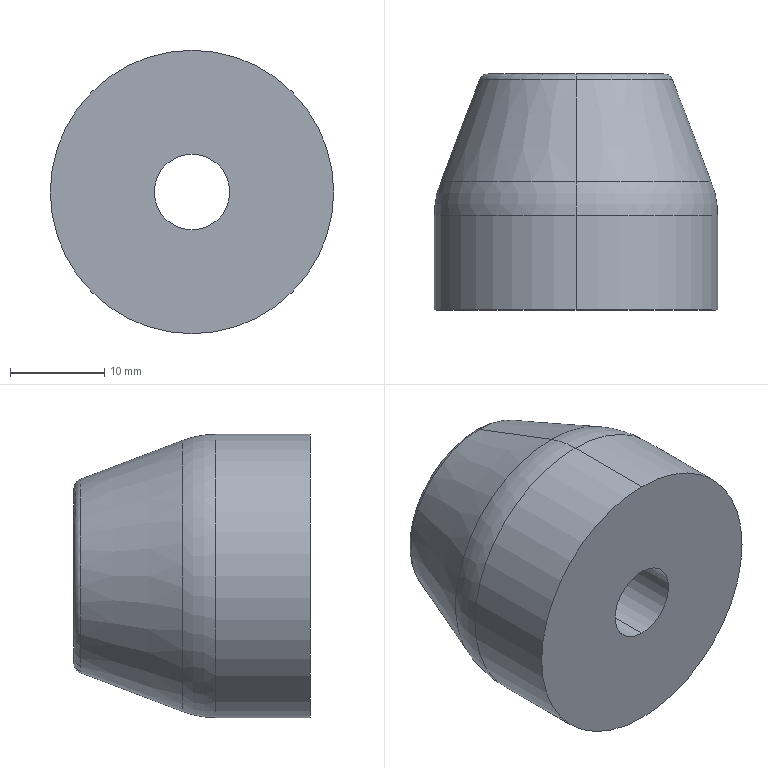Part | SolidWorks | features Revolution 1 | 1 solid | 15 faces | box 30 x 25 x 30 mm | volume 12754 mm3 | cylinder 6 | torus 4 | plane 3 | cone 2 | commonest cylinder face diameters 8 x2 12 x2 30 x2
STEP:
#1=CARTESIAN_POINT('',(0.,11.,4.));
#2=VERTEX_POINT('',#1);
#3=CARTESIAN_POINT('',(0.,11.,-4.));
#4=VERTEX_POINT('',#3);
#5=CARTESIAN_POINT('',(0.,11.,0.));
#6=DIRECTION('',(0.,-1.,0.));
#7=DIRECTION('',(0.,0.,-1.));
#8=AXIS2_PLACEMENT_3D('',#5,#6,#7);
#9=CIRCLE('',#8,4.);
#10=EDGE_CURVE('',#2,#4,#9,.T.);
#11=ORIENTED_EDGE('',*,*,#10,.F.);
#12=CARTESIAN_POINT('',(0.,0.,4.));
#13=VERTEX_POINT('',#12);
#14=CARTESIAN_POINT('',(0.,0.,4.));
#15=DIRECTION('',(0.,-1.,0.));
#16=VECTOR('',#15,1000.);
#17=LINE('',#14,#16);
#18=EDGE_CURVE('',#2,#13,#17,.T.);
#19=ORIENTED_EDGE('',*,*,#18,.T.);
#20=CARTESIAN_POINT('',(0.,0.,-4.));
#21=VERTEX_POINT('',#20);
#22=CARTESIAN_POINT('',(0.,0.,0.));
#23=DIRECTION('',(0.,-1.,0.));
#24=DIRECTION('',(0.,0.,-1.));
#25=AXIS2_PLACEMENT_3D('',#22,#23,#24);
#26=CIRCLE('',#25,4.);
#27=EDGE_CURVE('',#13,#21,#26,.T.);
#28=ORIENTED_EDGE('',*,*,#27,.T.);
#29=CARTESIAN_POINT('',(0.,0.,-4.));
#30=DIRECTION('',(0.,-1.,0.));
#31=VECTOR('',#30,1000.);
#32=LINE('',#29,#31);
#33=EDGE_CURVE('',#4,#21,#32,.T.);
#34=ORIENTED_EDGE('',*,*,#33,.F.);
#35=EDGE_LOOP('',(#11,#19,#28,#34));
#36=FACE_OUTER_BOUND('',#35,.T.);
#37=CARTESIAN_POINT('',(0.,0.,0.));
#38=DIRECTION('',(0.,-1.,0.));
#39=DIRECTION('',(0.,0.,-1.));
#40=AXIS2_PLACEMENT_3D('',#37,#38,#39);
#41=CYLINDRICAL_SURFACE('',#40,4.);
#42=ADVANCED_FACE('',(#36),#41,.F.);
#43=CARTESIAN_POINT('',(0.,10.,-15.));
#44=VERTEX_POINT('',#43);
#45=CARTESIAN_POINT('',(0.,10.,15.));
#46=VERTEX_POINT('',#45);
#47=CARTESIAN_POINT('',(0.,10.,0.));
#48=DIRECTION('',(0.,-1.,0.));
#49=DIRECTION('',(0.,0.,-1.));
#50=AXIS2_PLACEMENT_3D('',#47,#48,#49);
#51=CIRCLE('',#50,15.);
#52=EDGE_CURVE('',#44,#46,#51,.T.);
#53=ORIENTED_EDGE('',*,*,#52,.T.);
#54=CARTESIAN_POINT('',(0.,0.,15.));
#55=VERTEX_POINT('',#54);
#56=CARTESIAN_POINT('',(0.,0.,15.));
#57=DIRECTION('',(0.,-1.,0.));
#58=VECTOR('',#57,1000.);
#59=LINE('',#56,#58);
#60=EDGE_CURVE('',#46,#55,#59,.T.);
#61=ORIENTED_EDGE('',*,*,#60,.T.);
#62=CARTESIAN_POINT('',(0.,0.,-15.));
#63=VERTEX_POINT('',#62);
#64=CARTESIAN_POINT('',(0.,0.,0.));
#65=DIRECTION('',(0.,-1.,0.));
#66=DIRECTION('',(0.,0.,-1.));
#67=AXIS2_PLACEMENT_3D('',#64,#65,#66);
#68=CIRCLE('',#67,15.);
#69=EDGE_CURVE('',#63,#55,#68,.T.);
#70=ORIENTED_EDGE('',*,*,#69,.F.);
#71=CARTESIAN_POINT('',(0.,0.,-15.));
#72=DIRECTION('',(0.,-1.,0.));
#73=VECTOR('',#72,1000.);
#74=LINE('',#71,#73);
#75=EDGE_CURVE('',#44,#63,#74,.T.);
#76=ORIENTED_EDGE('',*,*,#75,.F.);
#77=EDGE_LOOP('',(#53,#61,#70,#76));
#78=FACE_OUTER_BOUND('',#77,.T.);
#79=CARTESIAN_POINT('',(0.,0.,0.));
#80=DIRECTION('',(0.,-1.,0.));
#81=DIRECTION('',(0.,0.,-1.));
#82=AXIS2_PLACEMENT_3D('',#79,#80,#81);
#83=CYLINDRICAL_SURFACE('',#82,15.);
#84=ADVANCED_FACE('',(#78),#83,.T.);
#85=CARTESIAN_POINT('',(0.,13.551,-14.348));
#86=VERTEX_POINT('',#85);
#87=CARTESIAN_POINT('',(0.,13.551,14.348));
#88=VERTEX_POINT('',#87);
#89=CARTESIAN_POINT('',(0.,13.551,0.));
#90=DIRECTION('',(0.,-1.,0.));
#91=DIRECTION('',(0.,0.,-1.));
#92=AXIS2_PLACEMENT_3D('',#89,#90,#91);
#93=CIRCLE('',#92,14.348);
#94=EDGE_CURVE('',#86,#88,#93,.T.);
#95=ORIENTED_EDGE('',*,*,#94,.T.);
#96=CARTESIAN_POINT('',(0.,10.,5.));
#97=DIRECTION('',(1.,0.,0.));
#98=DIRECTION('',(0.,0.,-1.));
#99=AXIS2_PLACEMENT_3D('',#96,#97,#98);
#100=CIRCLE('',#99,10.);
#101=EDGE_CURVE('',#88,#46,#100,.T.);
#102=ORIENTED_EDGE('',*,*,#101,.T.);
#103=ORIENTED_EDGE('',*,*,#52,.F.);
#104=CARTESIAN_POINT('',(0.,10.,-5.));
#105=DIRECTION('',(-1.,0.,0.));
#106=DIRECTION('',(0.,0.,1.));
#107=AXIS2_PLACEMENT_3D('',#104,#105,#106);
#108=CIRCLE('',#107,10.);
#109=EDGE_CURVE('',#86,#44,#108,.T.);
#110=ORIENTED_EDGE('',*,*,#109,.F.);
#111=EDGE_LOOP('',(#95,#102,#103,#110));
#112=FACE_OUTER_BOUND('',#111,.T.);
#113=CARTESIAN_POINT('',(0.,10.,0.));
#114=DIRECTION('',(0.,-1.,0.));
#115=DIRECTION('',(0.,0.,-1.));
#116=AXIS2_PLACEMENT_3D('',#113,#114,#115);
#117=TOROIDAL_SURFACE('',#116,5.,10.);
#118=ADVANCED_FACE('',(#112),#117,.T.);
#119=CARTESIAN_POINT('',(0.,24.355,-10.245));
#120=VERTEX_POINT('',#119);
#121=CARTESIAN_POINT('',(0.,24.355,10.245));
#122=VERTEX_POINT('',#121);
#123=CARTESIAN_POINT('',(0.,24.355,0.));
#124=DIRECTION('',(0.,-1.,0.));
#125=DIRECTION('',(0.,0.,-1.));
#126=AXIS2_PLACEMENT_3D('',#123,#124,#125);
#127=CIRCLE('',#126,10.245);
#128=EDGE_CURVE('',#120,#122,#127,.T.);
#129=ORIENTED_EDGE('',*,*,#128,.T.);
#130=CARTESIAN_POINT('',(0.,13.551,14.348));
#131=DIRECTION('',(0.,-0.9348,0.3551));
#132=VECTOR('',#131,1000.);
#133=LINE('',#130,#132);
#134=EDGE_CURVE('',#122,#88,#133,.T.);
#135=ORIENTED_EDGE('',*,*,#134,.T.);
#136=ORIENTED_EDGE('',*,*,#94,.F.);
#137=CARTESIAN_POINT('',(0.,13.551,-14.348));
#138=DIRECTION('',(0.,-0.9348,-0.3551));
#139=VECTOR('',#138,1000.);
#140=LINE('',#137,#139);
#141=EDGE_CURVE('',#120,#86,#140,.T.);
#142=ORIENTED_EDGE('',*,*,#141,.F.);
#143=EDGE_LOOP('',(#129,#135,#136,#142));
#144=FACE_OUTER_BOUND('',#143,.T.);
#145=CARTESIAN_POINT('',(0.,13.551,0.));
#146=DIRECTION('',(0.,-1.,0.));
#147=DIRECTION('',(0.,0.,-1.));
#148=AXIS2_PLACEMENT_3D('',#145,#146,#147);
#149=CONICAL_SURFACE('',#148,14.348,0.363);
#150=ADVANCED_FACE('',(#144),#149,.T.);
#151=CARTESIAN_POINT('',(0.,25.,-9.31));
#152=VERTEX_POINT('',#151);
#153=CARTESIAN_POINT('',(0.,25.,9.31));
#154=VERTEX_POINT('',#153);
#155=CARTESIAN_POINT('',(0.,25.,0.));
#156=DIRECTION('',(0.,-1.,0.));
#157=DIRECTION('',(0.,0.,-1.));
#158=AXIS2_PLACEMENT_3D('',#155,#156,#157);
#159=CIRCLE('',#158,9.31);
#160=EDGE_CURVE('',#152,#154,#159,.T.);
#161=ORIENTED_EDGE('',*,*,#160,.T.);
#162=CARTESIAN_POINT('',(0.,24.,9.31));
#163=DIRECTION('',(1.,0.,0.));
#164=DIRECTION('',(0.,0.,-1.));
#165=AXIS2_PLACEMENT_3D('',#162,#163,#164);
#166=CIRCLE('',#165,1.);
#167=EDGE_CURVE('',#154,#122,#166,.T.);
#168=ORIENTED_EDGE('',*,*,#167,.T.);
#169=ORIENTED_EDGE('',*,*,#128,.F.);
#170=CARTESIAN_POINT('',(0.,24.,-9.31));
#171=DIRECTION('',(-1.,0.,0.));
#172=DIRECTION('',(0.,0.,1.));
#173=AXIS2_PLACEMENT_3D('',#170,#171,#172);
#174=CIRCLE('',#173,1.);
#175=EDGE_CURVE('',#152,#120,#174,.T.);
#176=ORIENTED_EDGE('',*,*,#175,.F.);
#177=EDGE_LOOP('',(#161,#168,#169,#176));
#178=FACE_OUTER_BOUND('',#177,.T.);
#179=CARTESIAN_POINT('',(0.,24.,0.));
#180=DIRECTION('',(0.,-1.,0.));
#181=DIRECTION('',(0.,0.,-1.));
#182=AXIS2_PLACEMENT_3D('',#179,#180,#181);
#183=TOROIDAL_SURFACE('',#182,9.31,1.);
#184=ADVANCED_FACE('',(#178),#183,.T.);
#185=CARTESIAN_POINT('',(0.,25.,6.));
#186=VERTEX_POINT('',#185);
#187=CARTESIAN_POINT('',(0.,25.,-6.));
#188=VERTEX_POINT('',#187);
#189=CARTESIAN_POINT('',(0.,25.,0.));
#190=DIRECTION('',(0.,-1.,0.));
#191=DIRECTION('',(0.,0.,-1.));
#192=AXIS2_PLACEMENT_3D('',#189,#190,#191);
#193=CIRCLE('',#192,6.);
#194=EDGE_CURVE('',#186,#188,#193,.T.);
#195=ORIENTED_EDGE('',*,*,#194,.F.);
#196=CARTESIAN_POINT('',(0.,11.,6.));
#197=VERTEX_POINT('',#196);
#198=CARTESIAN_POINT('',(0.,0.,6.));
#199=DIRECTION('',(0.,-1.,0.));
#200=VECTOR('',#199,1000.);
#201=LINE('',#198,#200);
#202=EDGE_CURVE('',#186,#197,#201,.T.);
#203=ORIENTED_EDGE('',*,*,#202,.T.);
#204=CARTESIAN_POINT('',(0.,11.,-6.));
#205=VERTEX_POINT('',#204);
#206=CARTESIAN_POINT('',(0.,11.,0.));
#207=DIRECTION('',(0.,-1.,0.));
#208=DIRECTION('',(0.,0.,-1.));
#209=AXIS2_PLACEMENT_3D('',#206,#207,#208);
#210=CIRCLE('',#209,6.);
#211=EDGE_CURVE('',#197,#205,#210,.T.);
#212=ORIENTED_EDGE('',*,*,#211,.T.);
#213=CARTESIAN_POINT('',(0.,0.,-6.));
#214=DIRECTION('',(0.,-1.,0.));
#215=VECTOR('',#214,1000.);
#216=LINE('',#213,#215);
#217=EDGE_CURVE('',#188,#205,#216,.T.);
#218=ORIENTED_EDGE('',*,*,#217,.F.);
#219=EDGE_LOOP('',(#195,#203,#212,#218));
#220=FACE_OUTER_BOUND('',#219,.T.);
#221=CARTESIAN_POINT('',(0.,0.,0.));
#222=DIRECTION('',(0.,-1.,0.));
#223=DIRECTION('',(0.,0.,-1.));
#224=AXIS2_PLACEMENT_3D('',#221,#222,#223);
#225=CYLINDRICAL_SURFACE('',#224,6.);
#226=ADVANCED_FACE('',(#220),#225,.F.);
#227=ORIENTED_EDGE('',*,*,#202,.F.);
#228=CARTESIAN_POINT('',(0.,25.,0.));
#229=DIRECTION('',(0.,-1.,0.));
#230=DIRECTION('',(0.,0.,-1.));
#231=AXIS2_PLACEMENT_3D('',#228,#229,#230);
#232=CIRCLE('',#231,6.);
#233=EDGE_CURVE('',#188,#186,#232,.T.);
#234=ORIENTED_EDGE('',*,*,#233,.F.);
#235=ORIENTED_EDGE('',*,*,#217,.T.);
#236=CARTESIAN_POINT('',(0.,11.,0.));
#237=DIRECTION('',(0.,-1.,0.));
#238=DIRECTION('',(0.,0.,-1.));
#239=AXIS2_PLACEMENT_3D('',#236,#237,#238);
#240=CIRCLE('',#239,6.);
#241=EDGE_CURVE('',#205,#197,#240,.T.);
#242=ORIENTED_EDGE('',*,*,#241,.T.);
#243=EDGE_LOOP('',(#227,#234,#235,#242));
#244=FACE_OUTER_BOUND('',#243,.T.);
#245=CARTESIAN_POINT('',(0.,0.,0.));
#246=DIRECTION('',(0.,-1.,0.));
#247=DIRECTION('',(0.,0.,-1.));
#248=AXIS2_PLACEMENT_3D('',#245,#246,#247);
#249=CYLINDRICAL_SURFACE('',#248,6.);
#250=ADVANCED_FACE('',(#244),#249,.F.);
#251=ORIENTED_EDGE('',*,*,#233,.T.);
#252=ORIENTED_EDGE('',*,*,#194,.T.);
#253=EDGE_LOOP('',(#251,#252));
#254=FACE_BOUND('',#253,.T.);
#255=ORIENTED_EDGE('',*,*,#160,.F.);
#256=CARTESIAN_POINT('',(0.,25.,0.));
#257=DIRECTION('',(0.,-1.,0.));
#258=DIRECTION('',(0.,0.,-1.));
#259=AXIS2_PLACEMENT_3D('',#256,#257,#258);
#260=CIRCLE('',#259,9.31);
#261=EDGE_CURVE('',#154,#152,#260,.T.);
#262=ORIENTED_EDGE('',*,*,#261,.F.);
#263=EDGE_LOOP('',(#255,#262));
#264=FACE_OUTER_BOUND('',#263,.T.);
#265=CARTESIAN_POINT('',(6.,25.,0.));
#266=DIRECTION('',(0.,1.,0.));
#267=DIRECTION('',(0.,0.,1.));
#268=AXIS2_PLACEMENT_3D('',#265,#266,#267);
#269=PLANE('',#268);
#270=ADVANCED_FACE('',(#254,#264),#269,.T.);
#271=ORIENTED_EDGE('',*,*,#167,.F.);
#272=ORIENTED_EDGE('',*,*,#261,.T.);
#273=ORIENTED_EDGE('',*,*,#175,.T.);
#274=CARTESIAN_POINT('',(0.,24.355,0.));
#275=DIRECTION('',(0.,-1.,0.));
#276=DIRECTION('',(0.,0.,-1.));
#277=AXIS2_PLACEMENT_3D('',#274,#275,#276);
#278=CIRCLE('',#277,10.245);
#279=EDGE_CURVE('',#122,#120,#278,.T.);
#280=ORIENTED_EDGE('',*,*,#279,.F.);
#281=EDGE_LOOP('',(#271,#272,#273,#280));
#282=FACE_OUTER_BOUND('',#281,.T.);
#283=CARTESIAN_POINT('',(0.,24.,0.));
#284=DIRECTION('',(0.,-1.,0.));
#285=DIRECTION('',(0.,0.,-1.));
#286=AXIS2_PLACEMENT_3D('',#283,#284,#285);
#287=TOROIDAL_SURFACE('',#286,9.31,1.);
#288=ADVANCED_FACE('',(#282),#287,.T.);
#289=ORIENTED_EDGE('',*,*,#134,.F.);
#290=ORIENTED_EDGE('',*,*,#279,.T.);
#291=ORIENTED_EDGE('',*,*,#141,.T.);
#292=CARTESIAN_POINT('',(0.,13.551,0.));
#293=DIRECTION('',(0.,-1.,0.));
#294=DIRECTION('',(0.,0.,-1.));
#295=AXIS2_PLACEMENT_3D('',#292,#293,#294);
#296=CIRCLE('',#295,14.348);
#297=EDGE_CURVE('',#88,#86,#296,.T.);
#298=ORIENTED_EDGE('',*,*,#297,.F.);
#299=EDGE_LOOP('',(#289,#290,#291,#298));
#300=FACE_OUTER_BOUND('',#299,.T.);
#301=CARTESIAN_POINT('',(0.,13.551,0.));
#302=DIRECTION('',(0.,-1.,0.));
#303=DIRECTION('',(0.,0.,-1.));
#304=AXIS2_PLACEMENT_3D('',#301,#302,#303);
#305=CONICAL_SURFACE('',#304,14.348,0.363);
#306=ADVANCED_FACE('',(#300),#305,.T.);
#307=ORIENTED_EDGE('',*,*,#101,.F.);
#308=ORIENTED_EDGE('',*,*,#297,.T.);
#309=ORIENTED_EDGE('',*,*,#109,.T.);
#310=CARTESIAN_POINT('',(0.,10.,0.));
#311=DIRECTION('',(0.,-1.,0.));
#312=DIRECTION('',(0.,0.,-1.));
#313=AXIS2_PLACEMENT_3D('',#310,#311,#312);
#314=CIRCLE('',#313,15.);
#315=EDGE_CURVE('',#46,#44,#314,.T.);
#316=ORIENTED_EDGE('',*,*,#315,.F.);
#317=EDGE_LOOP('',(#307,#308,#309,#316));
#318=FACE_OUTER_BOUND('',#317,.T.);
#319=CARTESIAN_POINT('',(0.,10.,0.));
#320=DIRECTION('',(0.,-1.,0.));
#321=DIRECTION('',(0.,0.,-1.));
#322=AXIS2_PLACEMENT_3D('',#319,#320,#321);
#323=TOROIDAL_SURFACE('',#322,5.,10.);
#324=ADVANCED_FACE('',(#318),#323,.T.);
#325=ORIENTED_EDGE('',*,*,#60,.F.);
#326=ORIENTED_EDGE('',*,*,#315,.T.);
#327=ORIENTED_EDGE('',*,*,#75,.T.);
#328=CARTESIAN_POINT('',(0.,0.,0.));
#329=DIRECTION('',(0.,-1.,0.));
#330=DIRECTION('',(0.,0.,-1.));
#331=AXIS2_PLACEMENT_3D('',#328,#329,#330);
#332=CIRCLE('',#331,15.);
#333=EDGE_CURVE('',#55,#63,#332,.T.);
#334=ORIENTED_EDGE('',*,*,#333,.F.);
#335=EDGE_LOOP('',(#325,#326,#327,#334));
#336=FACE_OUTER_BOUND('',#335,.T.);
#337=CARTESIAN_POINT('',(0.,0.,0.));
#338=DIRECTION('',(0.,-1.,0.));
#339=DIRECTION('',(0.,0.,-1.));
#340=AXIS2_PLACEMENT_3D('',#337,#338,#339);
#341=CYLINDRICAL_SURFACE('',#340,15.);
#342=ADVANCED_FACE('',(#336),#341,.T.);
#343=ORIENTED_EDGE('',*,*,#69,.T.);
#344=ORIENTED_EDGE('',*,*,#333,.T.);
#345=EDGE_LOOP('',(#343,#344));
#346=FACE_OUTER_BOUND('',#345,.T.);
#347=CARTESIAN_POINT('',(0.,0.,0.));
#348=DIRECTION('',(0.,-1.,0.));
#349=DIRECTION('',(0.,0.,-1.));
#350=AXIS2_PLACEMENT_3D('',#347,#348,#349);
#351=CIRCLE('',#350,4.);
#352=EDGE_CURVE('',#21,#13,#351,.T.);
#353=ORIENTED_EDGE('',*,*,#352,.F.);
#354=ORIENTED_EDGE('',*,*,#27,.F.);
#355=EDGE_LOOP('',(#353,#354));
#356=FACE_BOUND('',#355,.T.);
#357=CARTESIAN_POINT('',(15.,0.,0.));
#358=DIRECTION('',(0.,-1.,0.));
#359=DIRECTION('',(0.,0.,-1.));
#360=AXIS2_PLACEMENT_3D('',#357,#358,#359);
#361=PLANE('',#360);
#362=ADVANCED_FACE('',(#346,#356),#361,.T.);
#363=ORIENTED_EDGE('',*,*,#18,.F.);
#364=CARTESIAN_POINT('',(0.,11.,0.));
#365=DIRECTION('',(0.,-1.,0.));
#366=DIRECTION('',(0.,0.,-1.));
#367=AXIS2_PLACEMENT_3D('',#364,#365,#366);
#368=CIRCLE('',#367,4.);
#369=EDGE_CURVE('',#4,#2,#368,.T.);
#370=ORIENTED_EDGE('',*,*,#369,.F.);
#371=ORIENTED_EDGE('',*,*,#33,.T.);
#372=ORIENTED_EDGE('',*,*,#352,.T.);
#373=EDGE_LOOP('',(#363,#370,#371,#372));
#374=FACE_OUTER_BOUND('',#373,.T.);
#375=CARTESIAN_POINT('',(0.,0.,0.));
#376=DIRECTION('',(0.,-1.,0.));
#377=DIRECTION('',(0.,0.,-1.));
#378=AXIS2_PLACEMENT_3D('',#375,#376,#377);
#379=CYLINDRICAL_SURFACE('',#378,4.);
#380=ADVANCED_FACE('',(#374),#379,.F.);
#381=ORIENTED_EDGE('',*,*,#369,.T.);
#382=ORIENTED_EDGE('',*,*,#10,.T.);
#383=EDGE_LOOP('',(#381,#382));
#384=FACE_BOUND('',#383,.T.);
#385=ORIENTED_EDGE('',*,*,#241,.F.);
#386=ORIENTED_EDGE('',*,*,#211,.F.);
#387=EDGE_LOOP('',(#385,#386));
#388=FACE_OUTER_BOUND('',#387,.T.);
#389=CARTESIAN_POINT('',(4.,11.,0.));
#390=DIRECTION('',(0.,1.,0.));
#391=DIRECTION('',(0.,0.,1.));
#392=AXIS2_PLACEMENT_3D('',#389,#390,#391);
#393=PLANE('',#392);
#394=ADVANCED_FACE('',(#384,#388),#393,.T.);
#395=CLOSED_SHELL('',(#42,#84,#118,#150,#184,#226,#250,#270,#288,#306,#324,#342,#362,#380,#394));
#396=MANIFOLD_SOLID_BREP('',#395);
#397=CARTESIAN_POINT('',(0.,0.,0.));
#398=DIRECTION('',(0.,0.,1.));
#399=DIRECTION('',(1.,0.,0.));
#400=AXIS2_PLACEMENT_3D('',#397,#398,#399);
#401=(LENGTH_UNIT()NAMED_UNIT(*)SI_UNIT(.MILLI.,.METRE.));
#402=UNCERTAINTY_MEASURE_WITH_UNIT(LENGTH_MEASURE(0.00001),#401,'','');
#403=(NAMED_UNIT(*)PLANE_ANGLE_UNIT()SI_UNIT($,.RADIAN.));
#404=(NAMED_UNIT(*)SI_UNIT($,.STERADIAN.)SOLID_ANGLE_UNIT());
#405=(GEOMETRIC_REPRESENTATION_CONTEXT(3)GLOBAL_UNCERTAINTY_ASSIGNED_CONTEXT((#402))GLOBAL_UNIT_ASSIGNED_CONTEXT((#401,#403,#404))REPRESENTATION_CONTEXT('',''));
#406=ADVANCED_BREP_SHAPE_REPRESENTATION('',(#396,#400),#405);